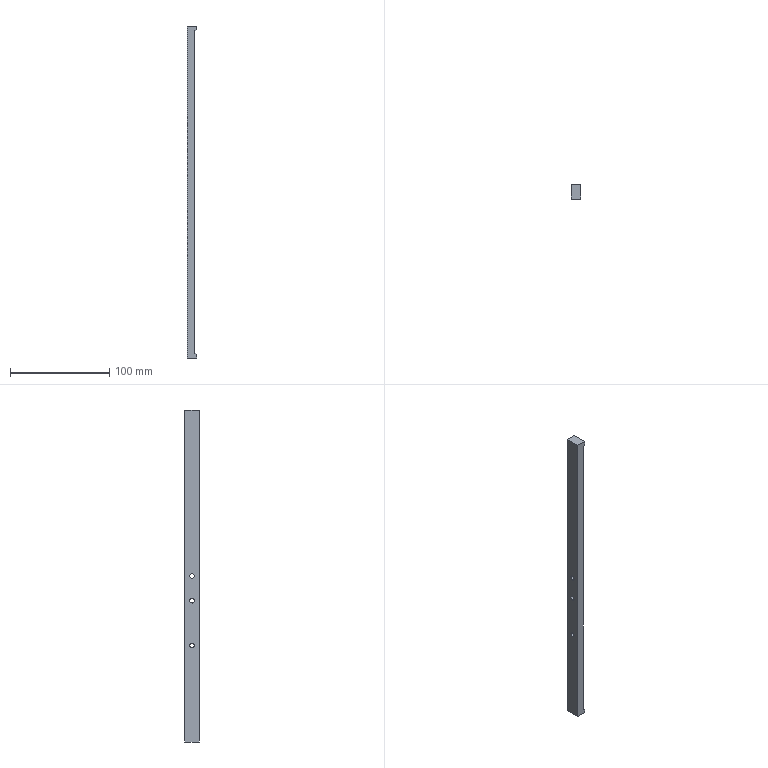Part | SolidWorks | features Extrusion 1, HoleWzd 1, ICE 1 | 1 solid | 25 faces | box 10 x 15 x 335 mm | volume 39599 mm3 | plane 13 | cylinder 12 | commonest cylinder face diameters 4.5 x6 8 x6
STEP:
#1=CARTESIAN_POINT('',(3.4,0.,4.));
#2=VERTEX_POINT('',#1);
#3=CARTESIAN_POINT('',(3.4,0.,-4.));
#4=VERTEX_POINT('',#3);
#5=CARTESIAN_POINT('',(3.4,0.,0.));
#6=DIRECTION('',(1.,0.,0.));
#7=DIRECTION('',(0.,0.,-1.));
#8=AXIS2_PLACEMENT_3D('',#5,#6,#7);
#9=CIRCLE('',#8,4.);
#10=EDGE_CURVE('',#2,#4,#9,.T.);
#11=ORIENTED_EDGE('',*,*,#10,.F.);
#12=CARTESIAN_POINT('',(8.,0.,4.));
#13=VERTEX_POINT('',#12);
#14=CARTESIAN_POINT('',(8.,0.,4.));
#15=DIRECTION('',(1.,0.,0.));
#16=VECTOR('',#15,1000.);
#17=LINE('',#14,#16);
#18=EDGE_CURVE('',#2,#13,#17,.T.);
#19=ORIENTED_EDGE('',*,*,#18,.T.);
#20=CARTESIAN_POINT('',(8.,0.,-4.));
#21=VERTEX_POINT('',#20);
#22=CARTESIAN_POINT('',(8.,0.,0.));
#23=DIRECTION('',(1.,0.,0.));
#24=DIRECTION('',(0.,0.,-1.));
#25=AXIS2_PLACEMENT_3D('',#22,#23,#24);
#26=CIRCLE('',#25,4.);
#27=EDGE_CURVE('',#13,#21,#26,.T.);
#28=ORIENTED_EDGE('',*,*,#27,.T.);
#29=CARTESIAN_POINT('',(8.,0.,-4.));
#30=DIRECTION('',(1.,0.,0.));
#31=VECTOR('',#30,1000.);
#32=LINE('',#29,#31);
#33=EDGE_CURVE('',#4,#21,#32,.T.);
#34=ORIENTED_EDGE('',*,*,#33,.F.);
#35=EDGE_LOOP('',(#11,#19,#28,#34));
#36=FACE_OUTER_BOUND('',#35,.T.);
#37=CARTESIAN_POINT('',(8.,0.,0.));
#38=DIRECTION('',(1.,0.,0.));
#39=DIRECTION('',(0.,0.,-1.));
#40=AXIS2_PLACEMENT_3D('',#37,#38,#39);
#41=CYLINDRICAL_SURFACE('',#40,4.);
#42=ADVANCED_FACE('',(#36),#41,.F.);
#43=CARTESIAN_POINT('',(0.,0.,2.25));
#44=VERTEX_POINT('',#43);
#45=CARTESIAN_POINT('',(0.,0.,-2.25));
#46=VERTEX_POINT('',#45);
#47=CARTESIAN_POINT('',(0.,0.,0.));
#48=DIRECTION('',(1.,0.,0.));
#49=DIRECTION('',(0.,0.,-1.));
#50=AXIS2_PLACEMENT_3D('',#47,#48,#49);
#51=CIRCLE('',#50,2.25);
#52=EDGE_CURVE('',#44,#46,#51,.T.);
#53=ORIENTED_EDGE('',*,*,#52,.F.);
#54=CARTESIAN_POINT('',(3.4,0.,2.25));
#55=VERTEX_POINT('',#54);
#56=CARTESIAN_POINT('',(8.,0.,2.25));
#57=DIRECTION('',(1.,0.,0.));
#58=VECTOR('',#57,1000.);
#59=LINE('',#56,#58);
#60=EDGE_CURVE('',#44,#55,#59,.T.);
#61=ORIENTED_EDGE('',*,*,#60,.T.);
#62=CARTESIAN_POINT('',(3.4,0.,-2.25));
#63=VERTEX_POINT('',#62);
#64=CARTESIAN_POINT('',(3.4,0.,0.));
#65=DIRECTION('',(1.,0.,0.));
#66=DIRECTION('',(0.,0.,-1.));
#67=AXIS2_PLACEMENT_3D('',#64,#65,#66);
#68=CIRCLE('',#67,2.25);
#69=EDGE_CURVE('',#55,#63,#68,.T.);
#70=ORIENTED_EDGE('',*,*,#69,.T.);
#71=CARTESIAN_POINT('',(8.,0.,-2.25));
#72=DIRECTION('',(1.,0.,0.));
#73=VECTOR('',#72,1000.);
#74=LINE('',#71,#73);
#75=EDGE_CURVE('',#46,#63,#74,.T.);
#76=ORIENTED_EDGE('',*,*,#75,.F.);
#77=EDGE_LOOP('',(#53,#61,#70,#76));
#78=FACE_OUTER_BOUND('',#77,.T.);
#79=CARTESIAN_POINT('',(8.,0.,0.));
#80=DIRECTION('',(1.,0.,0.));
#81=DIRECTION('',(0.,0.,-1.));
#82=AXIS2_PLACEMENT_3D('',#79,#80,#81);
#83=CYLINDRICAL_SURFACE('',#82,2.25);
#84=ADVANCED_FACE('',(#78),#83,.F.);
#85=CARTESIAN_POINT('',(3.4,0.,-66.));
#86=VERTEX_POINT('',#85);
#87=CARTESIAN_POINT('',(3.4,0.,-74.));
#88=VERTEX_POINT('',#87);
#89=CARTESIAN_POINT('',(3.4,0.,-70.));
#90=DIRECTION('',(1.,0.,0.));
#91=DIRECTION('',(0.,0.,-1.));
#92=AXIS2_PLACEMENT_3D('',#89,#90,#91);
#93=CIRCLE('',#92,4.);
#94=EDGE_CURVE('',#86,#88,#93,.T.);
#95=ORIENTED_EDGE('',*,*,#94,.F.);
#96=CARTESIAN_POINT('',(8.,0.,-66.));
#97=VERTEX_POINT('',#96);
#98=CARTESIAN_POINT('',(8.,0.,-66.));
#99=DIRECTION('',(1.,0.,0.));
#100=VECTOR('',#99,1000.);
#101=LINE('',#98,#100);
#102=EDGE_CURVE('',#86,#97,#101,.T.);
#103=ORIENTED_EDGE('',*,*,#102,.T.);
#104=CARTESIAN_POINT('',(8.,0.,-74.));
#105=VERTEX_POINT('',#104);
#106=CARTESIAN_POINT('',(8.,0.,-70.));
#107=DIRECTION('',(1.,0.,0.));
#108=DIRECTION('',(0.,0.,-1.));
#109=AXIS2_PLACEMENT_3D('',#106,#107,#108);
#110=CIRCLE('',#109,4.);
#111=EDGE_CURVE('',#97,#105,#110,.T.);
#112=ORIENTED_EDGE('',*,*,#111,.T.);
#113=CARTESIAN_POINT('',(8.,0.,-74.));
#114=DIRECTION('',(1.,0.,0.));
#115=VECTOR('',#114,1000.);
#116=LINE('',#113,#115);
#117=EDGE_CURVE('',#88,#105,#116,.T.);
#118=ORIENTED_EDGE('',*,*,#117,.F.);
#119=EDGE_LOOP('',(#95,#103,#112,#118));
#120=FACE_OUTER_BOUND('',#119,.T.);
#121=CARTESIAN_POINT('',(8.,0.,-70.));
#122=DIRECTION('',(1.,0.,0.));
#123=DIRECTION('',(0.,0.,-1.));
#124=AXIS2_PLACEMENT_3D('',#121,#122,#123);
#125=CYLINDRICAL_SURFACE('',#124,4.);
#126=ADVANCED_FACE('',(#120),#125,.F.);
#127=CARTESIAN_POINT('',(0.,0.,-67.75));
#128=VERTEX_POINT('',#127);
#129=CARTESIAN_POINT('',(0.,0.,-72.25));
#130=VERTEX_POINT('',#129);
#131=CARTESIAN_POINT('',(0.,0.,-70.));
#132=DIRECTION('',(1.,0.,0.));
#133=DIRECTION('',(0.,0.,-1.));
#134=AXIS2_PLACEMENT_3D('',#131,#132,#133);
#135=CIRCLE('',#134,2.25);
#136=EDGE_CURVE('',#128,#130,#135,.T.);
#137=ORIENTED_EDGE('',*,*,#136,.F.);
#138=CARTESIAN_POINT('',(3.4,0.,-67.75));
#139=VERTEX_POINT('',#138);
#140=CARTESIAN_POINT('',(8.,0.,-67.75));
#141=DIRECTION('',(1.,0.,0.));
#142=VECTOR('',#141,1000.);
#143=LINE('',#140,#142);
#144=EDGE_CURVE('',#128,#139,#143,.T.);
#145=ORIENTED_EDGE('',*,*,#144,.T.);
#146=CARTESIAN_POINT('',(3.4,0.,-72.25));
#147=VERTEX_POINT('',#146);
#148=CARTESIAN_POINT('',(3.4,0.,-70.));
#149=DIRECTION('',(1.,0.,0.));
#150=DIRECTION('',(0.,0.,-1.));
#151=AXIS2_PLACEMENT_3D('',#148,#149,#150);
#152=CIRCLE('',#151,2.25);
#153=EDGE_CURVE('',#139,#147,#152,.T.);
#154=ORIENTED_EDGE('',*,*,#153,.T.);
#155=CARTESIAN_POINT('',(8.,0.,-72.25));
#156=DIRECTION('',(1.,0.,0.));
#157=VECTOR('',#156,1000.);
#158=LINE('',#155,#157);
#159=EDGE_CURVE('',#130,#147,#158,.T.);
#160=ORIENTED_EDGE('',*,*,#159,.F.);
#161=EDGE_LOOP('',(#137,#145,#154,#160));
#162=FACE_OUTER_BOUND('',#161,.T.);
#163=CARTESIAN_POINT('',(8.,0.,-70.));
#164=DIRECTION('',(1.,0.,0.));
#165=DIRECTION('',(0.,0.,-1.));
#166=AXIS2_PLACEMENT_3D('',#163,#164,#165);
#167=CYLINDRICAL_SURFACE('',#166,2.25);
#168=ADVANCED_FACE('',(#162),#167,.F.);
#169=CARTESIAN_POINT('',(3.4,0.,-21.));
#170=VERTEX_POINT('',#169);
#171=CARTESIAN_POINT('',(3.4,0.,-29.));
#172=VERTEX_POINT('',#171);
#173=CARTESIAN_POINT('',(3.4,0.,-25.));
#174=DIRECTION('',(1.,0.,0.));
#175=DIRECTION('',(0.,0.,-1.));
#176=AXIS2_PLACEMENT_3D('',#173,#174,#175);
#177=CIRCLE('',#176,4.);
#178=EDGE_CURVE('',#170,#172,#177,.T.);
#179=ORIENTED_EDGE('',*,*,#178,.F.);
#180=CARTESIAN_POINT('',(8.,0.,-21.));
#181=VERTEX_POINT('',#180);
#182=CARTESIAN_POINT('',(8.,0.,-21.));
#183=DIRECTION('',(1.,0.,0.));
#184=VECTOR('',#183,1000.);
#185=LINE('',#182,#184);
#186=EDGE_CURVE('',#170,#181,#185,.T.);
#187=ORIENTED_EDGE('',*,*,#186,.T.);
#188=CARTESIAN_POINT('',(8.,0.,-29.));
#189=VERTEX_POINT('',#188);
#190=CARTESIAN_POINT('',(8.,0.,-25.));
#191=DIRECTION('',(1.,0.,0.));
#192=DIRECTION('',(0.,0.,-1.));
#193=AXIS2_PLACEMENT_3D('',#190,#191,#192);
#194=CIRCLE('',#193,4.);
#195=EDGE_CURVE('',#181,#189,#194,.T.);
#196=ORIENTED_EDGE('',*,*,#195,.T.);
#197=CARTESIAN_POINT('',(8.,0.,-29.));
#198=DIRECTION('',(1.,0.,0.));
#199=VECTOR('',#198,1000.);
#200=LINE('',#197,#199);
#201=EDGE_CURVE('',#172,#189,#200,.T.);
#202=ORIENTED_EDGE('',*,*,#201,.F.);
#203=EDGE_LOOP('',(#179,#187,#196,#202));
#204=FACE_OUTER_BOUND('',#203,.T.);
#205=CARTESIAN_POINT('',(8.,0.,-25.));
#206=DIRECTION('',(1.,0.,0.));
#207=DIRECTION('',(0.,0.,-1.));
#208=AXIS2_PLACEMENT_3D('',#205,#206,#207);
#209=CYLINDRICAL_SURFACE('',#208,4.);
#210=ADVANCED_FACE('',(#204),#209,.F.);
#211=CARTESIAN_POINT('',(0.,0.,-22.75));
#212=VERTEX_POINT('',#211);
#213=CARTESIAN_POINT('',(0.,0.,-27.25));
#214=VERTEX_POINT('',#213);
#215=CARTESIAN_POINT('',(0.,0.,-25.));
#216=DIRECTION('',(1.,0.,0.));
#217=DIRECTION('',(0.,0.,-1.));
#218=AXIS2_PLACEMENT_3D('',#215,#216,#217);
#219=CIRCLE('',#218,2.25);
#220=EDGE_CURVE('',#212,#214,#219,.T.);
#221=ORIENTED_EDGE('',*,*,#220,.F.);
#222=CARTESIAN_POINT('',(3.4,0.,-22.75));
#223=VERTEX_POINT('',#222);
#224=CARTESIAN_POINT('',(8.,0.,-22.75));
#225=DIRECTION('',(1.,0.,0.));
#226=VECTOR('',#225,1000.);
#227=LINE('',#224,#226);
#228=EDGE_CURVE('',#212,#223,#227,.T.);
#229=ORIENTED_EDGE('',*,*,#228,.T.);
#230=CARTESIAN_POINT('',(3.4,0.,-27.25));
#231=VERTEX_POINT('',#230);
#232=CARTESIAN_POINT('',(3.4,0.,-25.));
#233=DIRECTION('',(1.,0.,0.));
#234=DIRECTION('',(0.,0.,-1.));
#235=AXIS2_PLACEMENT_3D('',#232,#233,#234);
#236=CIRCLE('',#235,2.25);
#237=EDGE_CURVE('',#223,#231,#236,.T.);
#238=ORIENTED_EDGE('',*,*,#237,.T.);
#239=CARTESIAN_POINT('',(8.,0.,-27.25));
#240=DIRECTION('',(1.,0.,0.));
#241=VECTOR('',#240,1000.);
#242=LINE('',#239,#241);
#243=EDGE_CURVE('',#214,#231,#242,.T.);
#244=ORIENTED_EDGE('',*,*,#243,.F.);
#245=EDGE_LOOP('',(#221,#229,#238,#244));
#246=FACE_OUTER_BOUND('',#245,.T.);
#247=CARTESIAN_POINT('',(8.,0.,-25.));
#248=DIRECTION('',(1.,0.,0.));
#249=DIRECTION('',(0.,0.,-1.));
#250=AXIS2_PLACEMENT_3D('',#247,#248,#249);
#251=CYLINDRICAL_SURFACE('',#250,2.25);
#252=ADVANCED_FACE('',(#246),#251,.F.);
#253=CARTESIAN_POINT('',(10.,7.5,-167.5));
#254=VERTEX_POINT('',#253);
#255=CARTESIAN_POINT('',(10.,7.5,-164.));
#256=VERTEX_POINT('',#255);
#257=CARTESIAN_POINT('',(10.,7.5,167.5));
#258=DIRECTION('',(0.,0.,1.));
#259=VECTOR('',#258,1000.);
#260=LINE('',#257,#259);
#261=EDGE_CURVE('',#254,#256,#260,.T.);
#262=ORIENTED_EDGE('',*,*,#261,.T.);
#263=CARTESIAN_POINT('',(10.,-7.5,-164.));
#264=VERTEX_POINT('',#263);
#265=CARTESIAN_POINT('',(10.,7.5,-164.));
#266=DIRECTION('',(0.,-1.,0.));
#267=VECTOR('',#266,1000.);
#268=LINE('',#265,#267);
#269=EDGE_CURVE('',#256,#264,#268,.T.);
#270=ORIENTED_EDGE('',*,*,#269,.T.);
#271=CARTESIAN_POINT('',(10.,-7.5,-167.5));
#272=VERTEX_POINT('',#271);
#273=CARTESIAN_POINT('',(10.,-7.5,167.5));
#274=DIRECTION('',(0.,0.,-1.));
#275=VECTOR('',#274,1000.);
#276=LINE('',#273,#275);
#277=EDGE_CURVE('',#264,#272,#276,.T.);
#278=ORIENTED_EDGE('',*,*,#277,.T.);
#279=CARTESIAN_POINT('',(10.,-7.5,-167.5));
#280=DIRECTION('',(0.,1.,0.));
#281=VECTOR('',#280,1000.);
#282=LINE('',#279,#281);
#283=EDGE_CURVE('',#272,#254,#282,.T.);
#284=ORIENTED_EDGE('',*,*,#283,.T.);
#285=EDGE_LOOP('',(#262,#270,#278,#284));
#286=FACE_OUTER_BOUND('',#285,.T.);
#287=CARTESIAN_POINT('',(10.,0.,0.));
#288=DIRECTION('',(-1.,0.,0.));
#289=DIRECTION('',(0.,0.,1.));
#290=AXIS2_PLACEMENT_3D('',#287,#288,#289);
#291=PLANE('',#290);
#292=ADVANCED_FACE('',(#286),#291,.F.);
#293=CARTESIAN_POINT('',(0.,-7.5,-167.5));
#294=VERTEX_POINT('',#293);
#295=CARTESIAN_POINT('',(0.,7.5,-167.5));
#296=VERTEX_POINT('',#295);
#297=CARTESIAN_POINT('',(0.,-7.5,-167.5));
#298=DIRECTION('',(0.,1.,0.));
#299=VECTOR('',#298,1000.);
#300=LINE('',#297,#299);
#301=EDGE_CURVE('',#294,#296,#300,.T.);
#302=ORIENTED_EDGE('',*,*,#301,.T.);
#303=CARTESIAN_POINT('',(10.,7.5,-167.5));
#304=DIRECTION('',(-1.,0.,0.));
#305=VECTOR('',#304,1000.);
#306=LINE('',#303,#305);
#307=EDGE_CURVE('',#254,#296,#306,.T.);
#308=ORIENTED_EDGE('',*,*,#307,.F.);
#309=ORIENTED_EDGE('',*,*,#283,.F.);
#310=CARTESIAN_POINT('',(10.,-7.5,-167.5));
#311=DIRECTION('',(-1.,0.,0.));
#312=VECTOR('',#311,1000.);
#313=LINE('',#310,#312);
#314=EDGE_CURVE('',#272,#294,#313,.T.);
#315=ORIENTED_EDGE('',*,*,#314,.T.);
#316=EDGE_LOOP('',(#302,#308,#309,#315));
#317=FACE_OUTER_BOUND('',#316,.T.);
#318=CARTESIAN_POINT('',(10.,-7.5,-167.5));
#319=DIRECTION('',(0.,0.,1.));
#320=DIRECTION('',(1.,0.,0.));
#321=AXIS2_PLACEMENT_3D('',#318,#319,#320);
#322=PLANE('',#321);
#323=ADVANCED_FACE('',(#317),#322,.F.);
#324=CARTESIAN_POINT('',(8.,7.5,162.5));
#325=VERTEX_POINT('',#324);
#326=CARTESIAN_POINT('',(8.,7.5,-162.5));
#327=VERTEX_POINT('',#326);
#328=CARTESIAN_POINT('',(8.,7.5,162.5));
#329=DIRECTION('',(0.,0.,-1.));
#330=VECTOR('',#329,1000.);
#331=LINE('',#328,#330);
#332=EDGE_CURVE('',#325,#327,#331,.T.);
#333=ORIENTED_EDGE('',*,*,#332,.T.);
#334=CARTESIAN_POINT('',(10.,7.5,-164.));
#335=DIRECTION('',(0.8,0.,-0.6));
#336=VECTOR('',#335,1000.);
#337=LINE('',#334,#336);
#338=EDGE_CURVE('',#327,#256,#337,.T.);
#339=ORIENTED_EDGE('',*,*,#338,.T.);
#340=ORIENTED_EDGE('',*,*,#261,.F.);
#341=ORIENTED_EDGE('',*,*,#307,.T.);
#342=CARTESIAN_POINT('',(0.,7.5,167.5));
#343=VERTEX_POINT('',#342);
#344=CARTESIAN_POINT('',(0.,7.5,167.5));
#345=DIRECTION('',(0.,0.,1.));
#346=VECTOR('',#345,1000.);
#347=LINE('',#344,#346);
#348=EDGE_CURVE('',#296,#343,#347,.T.);
#349=ORIENTED_EDGE('',*,*,#348,.T.);
#350=CARTESIAN_POINT('',(10.,7.5,167.5));
#351=VERTEX_POINT('',#350);
#352=CARTESIAN_POINT('',(10.,7.5,167.5));
#353=DIRECTION('',(-1.,0.,0.));
#354=VECTOR('',#353,1000.);
#355=LINE('',#352,#354);
#356=EDGE_CURVE('',#351,#343,#355,.T.);
#357=ORIENTED_EDGE('',*,*,#356,.F.);
#358=CARTESIAN_POINT('',(10.,7.5,164.));
#359=VERTEX_POINT('',#358);
#360=CARTESIAN_POINT('',(10.,7.5,167.5));
#361=DIRECTION('',(0.,0.,1.));
#362=VECTOR('',#361,1000.);
#363=LINE('',#360,#362);
#364=EDGE_CURVE('',#359,#351,#363,.T.);
#365=ORIENTED_EDGE('',*,*,#364,.F.);
#366=CARTESIAN_POINT('',(10.,7.5,164.));
#367=DIRECTION('',(-0.8,0.,-0.6));
#368=VECTOR('',#367,1000.);
#369=LINE('',#366,#368);
#370=EDGE_CURVE('',#359,#325,#369,.T.);
#371=ORIENTED_EDGE('',*,*,#370,.T.);
#372=EDGE_LOOP('',(#333,#339,#340,#341,#349,#357,#365,#371));
#373=FACE_OUTER_BOUND('',#372,.T.);
#374=CARTESIAN_POINT('',(10.,7.5,167.5));
#375=DIRECTION('',(0.,-1.,0.));
#376=DIRECTION('',(0.,0.,-1.));
#377=AXIS2_PLACEMENT_3D('',#374,#375,#376);
#378=PLANE('',#377);
#379=ADVANCED_FACE('',(#373),#378,.F.);
#380=CARTESIAN_POINT('',(0.,-7.5,167.5));
#381=VERTEX_POINT('',#380);
#382=CARTESIAN_POINT('',(0.,-7.5,167.5));
#383=DIRECTION('',(0.,-1.,0.));
#384=VECTOR('',#383,1000.);
#385=LINE('',#382,#384);
#386=EDGE_CURVE('',#343,#381,#385,.T.);
#387=ORIENTED_EDGE('',*,*,#386,.T.);
#388=CARTESIAN_POINT('',(10.,-7.5,167.5));
#389=VERTEX_POINT('',#388);
#390=CARTESIAN_POINT('',(10.,-7.5,167.5));
#391=DIRECTION('',(-1.,0.,0.));
#392=VECTOR('',#391,1000.);
#393=LINE('',#390,#392);
#394=EDGE_CURVE('',#389,#381,#393,.T.);
#395=ORIENTED_EDGE('',*,*,#394,.F.);
#396=CARTESIAN_POINT('',(10.,-7.5,167.5));
#397=DIRECTION('',(0.,-1.,0.));
#398=VECTOR('',#397,1000.);
#399=LINE('',#396,#398);
#400=EDGE_CURVE('',#351,#389,#399,.T.);
#401=ORIENTED_EDGE('',*,*,#400,.F.);
#402=ORIENTED_EDGE('',*,*,#356,.T.);
#403=EDGE_LOOP('',(#387,#395,#401,#402));
#404=FACE_OUTER_BOUND('',#403,.T.);
#405=CARTESIAN_POINT('',(10.,-7.5,167.5));
#406=DIRECTION('',(0.,0.,-1.));
#407=DIRECTION('',(-1.,0.,0.));
#408=AXIS2_PLACEMENT_3D('',#405,#406,#407);
#409=PLANE('',#408);
#410=ADVANCED_FACE('',(#404),#409,.F.);
#411=ORIENTED_EDGE('',*,*,#277,.F.);
#412=CARTESIAN_POINT('',(8.,-7.5,-162.5));
#413=VERTEX_POINT('',#412);
#414=CARTESIAN_POINT('',(10.,-7.5,-164.));
#415=DIRECTION('',(0.8,0.,-0.6));
#416=VECTOR('',#415,1000.);
#417=LINE('',#414,#416);
#418=EDGE_CURVE('',#413,#264,#417,.T.);
#419=ORIENTED_EDGE('',*,*,#418,.F.);
#420=CARTESIAN_POINT('',(8.,-7.5,162.5));
#421=VERTEX_POINT('',#420);
#422=CARTESIAN_POINT('',(8.,-7.5,162.5));
#423=DIRECTION('',(0.,0.,-1.));
#424=VECTOR('',#423,1000.);
#425=LINE('',#422,#424);
#426=EDGE_CURVE('',#421,#413,#425,.T.);
#427=ORIENTED_EDGE('',*,*,#426,.F.);
#428=CARTESIAN_POINT('',(10.,-7.5,164.));
#429=VERTEX_POINT('',#428);
#430=CARTESIAN_POINT('',(10.,-7.5,164.));
#431=DIRECTION('',(-0.8,0.,-0.6));
#432=VECTOR('',#431,1000.);
#433=LINE('',#430,#432);
#434=EDGE_CURVE('',#429,#421,#433,.T.);
#435=ORIENTED_EDGE('',*,*,#434,.F.);
#436=CARTESIAN_POINT('',(10.,-7.5,167.5));
#437=DIRECTION('',(0.,0.,-1.));
#438=VECTOR('',#437,1000.);
#439=LINE('',#436,#438);
#440=EDGE_CURVE('',#389,#429,#439,.T.);
#441=ORIENTED_EDGE('',*,*,#440,.F.);
#442=ORIENTED_EDGE('',*,*,#394,.T.);
#443=CARTESIAN_POINT('',(0.,-7.5,167.5));
#444=DIRECTION('',(0.,0.,-1.));
#445=VECTOR('',#444,1000.);
#446=LINE('',#443,#445);
#447=EDGE_CURVE('',#381,#294,#446,.T.);
#448=ORIENTED_EDGE('',*,*,#447,.T.);
#449=ORIENTED_EDGE('',*,*,#314,.F.);
#450=EDGE_LOOP('',(#411,#419,#427,#435,#441,#442,#448,#449));
#451=FACE_OUTER_BOUND('',#450,.T.);
#452=CARTESIAN_POINT('',(10.,-7.5,167.5));
#453=DIRECTION('',(0.,1.,0.));
#454=DIRECTION('',(0.,0.,1.));
#455=AXIS2_PLACEMENT_3D('',#452,#453,#454);
#456=PLANE('',#455);
#457=ADVANCED_FACE('',(#451),#456,.F.);
#458=ORIENTED_EDGE('',*,*,#440,.T.);
#459=CARTESIAN_POINT('',(10.,7.5,164.));
#460=DIRECTION('',(0.,-1.,0.));
#461=VECTOR('',#460,1000.);
#462=LINE('',#459,#461);
#463=EDGE_CURVE('',#359,#429,#462,.T.);
#464=ORIENTED_EDGE('',*,*,#463,.F.);
#465=ORIENTED_EDGE('',*,*,#364,.T.);
#466=ORIENTED_EDGE('',*,*,#400,.T.);
#467=EDGE_LOOP('',(#458,#464,#465,#466));
#468=FACE_OUTER_BOUND('',#467,.T.);
#469=CARTESIAN_POINT('',(10.,0.,0.));
#470=DIRECTION('',(-1.,0.,0.));
#471=DIRECTION('',(0.,0.,1.));
#472=AXIS2_PLACEMENT_3D('',#469,#470,#471);
#473=PLANE('',#472);
#474=ADVANCED_FACE('',(#468),#473,.F.);
#475=CARTESIAN_POINT('',(0.,0.,0.));
#476=DIRECTION('',(1.,0.,0.));
#477=DIRECTION('',(0.,0.,-1.));
#478=AXIS2_PLACEMENT_3D('',#475,#476,#477);
#479=CIRCLE('',#478,2.25);
#480=EDGE_CURVE('',#46,#44,#479,.T.);
#481=ORIENTED_EDGE('',*,*,#480,.T.);
#482=ORIENTED_EDGE('',*,*,#52,.T.);
#483=EDGE_LOOP('',(#481,#482));
#484=FACE_BOUND('',#483,.T.);
#485=CARTESIAN_POINT('',(0.,0.,-70.));
#486=DIRECTION('',(1.,0.,0.));
#487=DIRECTION('',(0.,0.,-1.));
#488=AXIS2_PLACEMENT_3D('',#485,#486,#487);
#489=CIRCLE('',#488,2.25);
#490=EDGE_CURVE('',#130,#128,#489,.T.);
#491=ORIENTED_EDGE('',*,*,#490,.T.);
#492=ORIENTED_EDGE('',*,*,#136,.T.);
#493=EDGE_LOOP('',(#491,#492));
#494=FACE_BOUND('',#493,.T.);
#495=CARTESIAN_POINT('',(0.,0.,-25.));
#496=DIRECTION('',(1.,0.,0.));
#497=DIRECTION('',(0.,0.,-1.));
#498=AXIS2_PLACEMENT_3D('',#495,#496,#497);
#499=CIRCLE('',#498,2.25);
#500=EDGE_CURVE('',#214,#212,#499,.T.);
#501=ORIENTED_EDGE('',*,*,#500,.T.);
#502=ORIENTED_EDGE('',*,*,#220,.T.);
#503=EDGE_LOOP('',(#501,#502));
#504=FACE_BOUND('',#503,.T.);
#505=ORIENTED_EDGE('',*,*,#301,.F.);
#506=ORIENTED_EDGE('',*,*,#447,.F.);
#507=ORIENTED_EDGE('',*,*,#386,.F.);
#508=ORIENTED_EDGE('',*,*,#348,.F.);
#509=EDGE_LOOP('',(#505,#506,#507,#508));
#510=FACE_OUTER_BOUND('',#509,.T.);
#511=CARTESIAN_POINT('',(0.,0.,0.));
#512=DIRECTION('',(-1.,0.,0.));
#513=DIRECTION('',(0.,0.,1.));
#514=AXIS2_PLACEMENT_3D('',#511,#512,#513);
#515=PLANE('',#514);
#516=ADVANCED_FACE('',(#484,#494,#504,#510),#515,.T.);
#517=ORIENTED_EDGE('',*,*,#418,.T.);
#518=ORIENTED_EDGE('',*,*,#269,.F.);
#519=ORIENTED_EDGE('',*,*,#338,.F.);
#520=CARTESIAN_POINT('',(8.,7.5,-162.5));
#521=DIRECTION('',(0.,-1.,0.));
#522=VECTOR('',#521,1000.);
#523=LINE('',#520,#522);
#524=EDGE_CURVE('',#327,#413,#523,.T.);
#525=ORIENTED_EDGE('',*,*,#524,.T.);
#526=EDGE_LOOP('',(#517,#518,#519,#525));
#527=FACE_OUTER_BOUND('',#526,.T.);
#528=CARTESIAN_POINT('',(10.,7.5,-164.));
#529=DIRECTION('',(-0.6,0.,-0.8));
#530=DIRECTION('',(-0.8,0.,0.6));
#531=AXIS2_PLACEMENT_3D('',#528,#529,#530);
#532=PLANE('',#531);
#533=ADVANCED_FACE('',(#527),#532,.F.);
#534=CARTESIAN_POINT('',(8.,0.,0.));
#535=DIRECTION('',(1.,0.,0.));
#536=DIRECTION('',(0.,0.,-1.));
#537=AXIS2_PLACEMENT_3D('',#534,#535,#536);
#538=CIRCLE('',#537,4.);
#539=EDGE_CURVE('',#21,#13,#538,.T.);
#540=ORIENTED_EDGE('',*,*,#539,.F.);
#541=ORIENTED_EDGE('',*,*,#27,.F.);
#542=EDGE_LOOP('',(#540,#541));
#543=FACE_BOUND('',#542,.T.);
#544=CARTESIAN_POINT('',(8.,0.,-70.));
#545=DIRECTION('',(1.,0.,0.));
#546=DIRECTION('',(0.,0.,-1.));
#547=AXIS2_PLACEMENT_3D('',#544,#545,#546);
#548=CIRCLE('',#547,4.);
#549=EDGE_CURVE('',#105,#97,#548,.T.);
#550=ORIENTED_EDGE('',*,*,#549,.F.);
#551=ORIENTED_EDGE('',*,*,#111,.F.);
#552=EDGE_LOOP('',(#550,#551));
#553=FACE_BOUND('',#552,.T.);
#554=CARTESIAN_POINT('',(8.,0.,-25.));
#555=DIRECTION('',(1.,0.,0.));
#556=DIRECTION('',(0.,0.,-1.));
#557=AXIS2_PLACEMENT_3D('',#554,#555,#556);
#558=CIRCLE('',#557,4.);
#559=EDGE_CURVE('',#189,#181,#558,.T.);
#560=ORIENTED_EDGE('',*,*,#559,.F.);
#561=ORIENTED_EDGE('',*,*,#195,.F.);
#562=EDGE_LOOP('',(#560,#561));
#563=FACE_BOUND('',#562,.T.);
#564=ORIENTED_EDGE('',*,*,#426,.T.);
#565=ORIENTED_EDGE('',*,*,#524,.F.);
#566=ORIENTED_EDGE('',*,*,#332,.F.);
#567=CARTESIAN_POINT('',(8.,7.5,162.5));
#568=DIRECTION('',(0.,-1.,0.));
#569=VECTOR('',#568,1000.);
#570=LINE('',#567,#569);
#571=EDGE_CURVE('',#325,#421,#570,.T.);
#572=ORIENTED_EDGE('',*,*,#571,.T.);
#573=EDGE_LOOP('',(#564,#565,#566,#572));
#574=FACE_OUTER_BOUND('',#573,.T.);
#575=CARTESIAN_POINT('',(8.,7.5,162.5));
#576=DIRECTION('',(-1.,0.,0.));
#577=DIRECTION('',(0.,0.,1.));
#578=AXIS2_PLACEMENT_3D('',#575,#576,#577);
#579=PLANE('',#578);
#580=ADVANCED_FACE('',(#543,#553,#563,#574),#579,.F.);
#581=ORIENTED_EDGE('',*,*,#434,.T.);
#582=ORIENTED_EDGE('',*,*,#571,.F.);
#583=ORIENTED_EDGE('',*,*,#370,.F.);
#584=ORIENTED_EDGE('',*,*,#463,.T.);
#585=EDGE_LOOP('',(#581,#582,#583,#584));
#586=FACE_OUTER_BOUND('',#585,.T.);
#587=CARTESIAN_POINT('',(10.,7.5,164.));
#588=DIRECTION('',(-0.6,0.,0.8));
#589=DIRECTION('',(0.8,0.,0.6));
#590=AXIS2_PLACEMENT_3D('',#587,#588,#589);
#591=PLANE('',#590);
#592=ADVANCED_FACE('',(#586),#591,.F.);
#593=ORIENTED_EDGE('',*,*,#228,.F.);
#594=ORIENTED_EDGE('',*,*,#500,.F.);
#595=ORIENTED_EDGE('',*,*,#243,.T.);
#596=CARTESIAN_POINT('',(3.4,0.,-25.));
#597=DIRECTION('',(1.,0.,0.));
#598=DIRECTION('',(0.,0.,-1.));
#599=AXIS2_PLACEMENT_3D('',#596,#597,#598);
#600=CIRCLE('',#599,2.25);
#601=EDGE_CURVE('',#231,#223,#600,.T.);
#602=ORIENTED_EDGE('',*,*,#601,.T.);
#603=EDGE_LOOP('',(#593,#594,#595,#602));
#604=FACE_OUTER_BOUND('',#603,.T.);
#605=CARTESIAN_POINT('',(8.,0.,-25.));
#606=DIRECTION('',(1.,0.,0.));
#607=DIRECTION('',(0.,0.,-1.));
#608=AXIS2_PLACEMENT_3D('',#605,#606,#607);
#609=CYLINDRICAL_SURFACE('',#608,2.25);
#610=ADVANCED_FACE('',(#604),#609,.F.);
#611=ORIENTED_EDGE('',*,*,#601,.F.);
#612=ORIENTED_EDGE('',*,*,#237,.F.);
#613=EDGE_LOOP('',(#611,#612));
#614=FACE_BOUND('',#613,.T.);
#615=CARTESIAN_POINT('',(3.4,0.,-25.));
#616=DIRECTION('',(1.,0.,0.));
#617=DIRECTION('',(0.,0.,-1.));
#618=AXIS2_PLACEMENT_3D('',#615,#616,#617);
#619=CIRCLE('',#618,4.);
#620=EDGE_CURVE('',#172,#170,#619,.T.);
#621=ORIENTED_EDGE('',*,*,#620,.T.);
#622=ORIENTED_EDGE('',*,*,#178,.T.);
#623=EDGE_LOOP('',(#621,#622));
#624=FACE_OUTER_BOUND('',#623,.T.);
#625=CARTESIAN_POINT('',(3.4,2.25,-25.));
#626=DIRECTION('',(-1.,0.,0.));
#627=DIRECTION('',(0.,0.,1.));
#628=AXIS2_PLACEMENT_3D('',#625,#626,#627);
#629=PLANE('',#628);
#630=ADVANCED_FACE('',(#614,#624),#629,.F.);
#631=ORIENTED_EDGE('',*,*,#186,.F.);
#632=ORIENTED_EDGE('',*,*,#620,.F.);
#633=ORIENTED_EDGE('',*,*,#201,.T.);
#634=ORIENTED_EDGE('',*,*,#559,.T.);
#635=EDGE_LOOP('',(#631,#632,#633,#634));
#636=FACE_OUTER_BOUND('',#635,.T.);
#637=CARTESIAN_POINT('',(8.,0.,-25.));
#638=DIRECTION('',(1.,0.,0.));
#639=DIRECTION('',(0.,0.,-1.));
#640=AXIS2_PLACEMENT_3D('',#637,#638,#639);
#641=CYLINDRICAL_SURFACE('',#640,4.);
#642=ADVANCED_FACE('',(#636),#641,.F.);
#643=ORIENTED_EDGE('',*,*,#144,.F.);
#644=ORIENTED_EDGE('',*,*,#490,.F.);
#645=ORIENTED_EDGE('',*,*,#159,.T.);
#646=CARTESIAN_POINT('',(3.4,0.,-70.));
#647=DIRECTION('',(1.,0.,0.));
#648=DIRECTION('',(0.,0.,-1.));
#649=AXIS2_PLACEMENT_3D('',#646,#647,#648);
#650=CIRCLE('',#649,2.25);
#651=EDGE_CURVE('',#147,#139,#650,.T.);
#652=ORIENTED_EDGE('',*,*,#651,.T.);
#653=EDGE_LOOP('',(#643,#644,#645,#652));
#654=FACE_OUTER_BOUND('',#653,.T.);
#655=CARTESIAN_POINT('',(8.,0.,-70.));
#656=DIRECTION('',(1.,0.,0.));
#657=DIRECTION('',(0.,0.,-1.));
#658=AXIS2_PLACEMENT_3D('',#655,#656,#657);
#659=CYLINDRICAL_SURFACE('',#658,2.25);
#660=ADVANCED_FACE('',(#654),#659,.F.);
#661=ORIENTED_EDGE('',*,*,#651,.F.);
#662=ORIENTED_EDGE('',*,*,#153,.F.);
#663=EDGE_LOOP('',(#661,#662));
#664=FACE_BOUND('',#663,.T.);
#665=CARTESIAN_POINT('',(3.4,0.,-70.));
#666=DIRECTION('',(1.,0.,0.));
#667=DIRECTION('',(0.,0.,-1.));
#668=AXIS2_PLACEMENT_3D('',#665,#666,#667);
#669=CIRCLE('',#668,4.);
#670=EDGE_CURVE('',#88,#86,#669,.T.);
#671=ORIENTED_EDGE('',*,*,#670,.T.);
#672=ORIENTED_EDGE('',*,*,#94,.T.);
#673=EDGE_LOOP('',(#671,#672));
#674=FACE_OUTER_BOUND('',#673,.T.);
#675=CARTESIAN_POINT('',(3.4,2.25,-70.));
#676=DIRECTION('',(-1.,0.,0.));
#677=DIRECTION('',(0.,0.,1.));
#678=AXIS2_PLACEMENT_3D('',#675,#676,#677);
#679=PLANE('',#678);
#680=ADVANCED_FACE('',(#664,#674),#679,.F.);
#681=ORIENTED_EDGE('',*,*,#102,.F.);
#682=ORIENTED_EDGE('',*,*,#670,.F.);
#683=ORIENTED_EDGE('',*,*,#117,.T.);
#684=ORIENTED_EDGE('',*,*,#549,.T.);
#685=EDGE_LOOP('',(#681,#682,#683,#684));
#686=FACE_OUTER_BOUND('',#685,.T.);
#687=CARTESIAN_POINT('',(8.,0.,-70.));
#688=DIRECTION('',(1.,0.,0.));
#689=DIRECTION('',(0.,0.,-1.));
#690=AXIS2_PLACEMENT_3D('',#687,#688,#689);
#691=CYLINDRICAL_SURFACE('',#690,4.);
#692=ADVANCED_FACE('',(#686),#691,.F.);
#693=ORIENTED_EDGE('',*,*,#60,.F.);
#694=ORIENTED_EDGE('',*,*,#480,.F.);
#695=ORIENTED_EDGE('',*,*,#75,.T.);
#696=CARTESIAN_POINT('',(3.4,0.,0.));
#697=DIRECTION('',(1.,0.,0.));
#698=DIRECTION('',(0.,0.,-1.));
#699=AXIS2_PLACEMENT_3D('',#696,#697,#698);
#700=CIRCLE('',#699,2.25);
#701=EDGE_CURVE('',#63,#55,#700,.T.);
#702=ORIENTED_EDGE('',*,*,#701,.T.);
#703=EDGE_LOOP('',(#693,#694,#695,#702));
#704=FACE_OUTER_BOUND('',#703,.T.);
#705=CARTESIAN_POINT('',(8.,0.,0.));
#706=DIRECTION('',(1.,0.,0.));
#707=DIRECTION('',(0.,0.,-1.));
#708=AXIS2_PLACEMENT_3D('',#705,#706,#707);
#709=CYLINDRICAL_SURFACE('',#708,2.25);
#710=ADVANCED_FACE('',(#704),#709,.F.);
#711=ORIENTED_EDGE('',*,*,#701,.F.);
#712=ORIENTED_EDGE('',*,*,#69,.F.);
#713=EDGE_LOOP('',(#711,#712));
#714=FACE_BOUND('',#713,.T.);
#715=CARTESIAN_POINT('',(3.4,0.,0.));
#716=DIRECTION('',(1.,0.,0.));
#717=DIRECTION('',(0.,0.,-1.));
#718=AXIS2_PLACEMENT_3D('',#715,#716,#717);
#719=CIRCLE('',#718,4.);
#720=EDGE_CURVE('',#4,#2,#719,.T.);
#721=ORIENTED_EDGE('',*,*,#720,.T.);
#722=ORIENTED_EDGE('',*,*,#10,.T.);
#723=EDGE_LOOP('',(#721,#722));
#724=FACE_OUTER_BOUND('',#723,.T.);
#725=CARTESIAN_POINT('',(3.4,2.25,0.));
#726=DIRECTION('',(-1.,0.,0.));
#727=DIRECTION('',(0.,0.,1.));
#728=AXIS2_PLACEMENT_3D('',#725,#726,#727);
#729=PLANE('',#728);
#730=ADVANCED_FACE('',(#714,#724),#729,.F.);
#731=ORIENTED_EDGE('',*,*,#18,.F.);
#732=ORIENTED_EDGE('',*,*,#720,.F.);
#733=ORIENTED_EDGE('',*,*,#33,.T.);
#734=ORIENTED_EDGE('',*,*,#539,.T.);
#735=EDGE_LOOP('',(#731,#732,#733,#734));
#736=FACE_OUTER_BOUND('',#735,.T.);
#737=CARTESIAN_POINT('',(8.,0.,0.));
#738=DIRECTION('',(1.,0.,0.));
#739=DIRECTION('',(0.,0.,-1.));
#740=AXIS2_PLACEMENT_3D('',#737,#738,#739);
#741=CYLINDRICAL_SURFACE('',#740,4.);
#742=ADVANCED_FACE('',(#736),#741,.F.);
#743=CLOSED_SHELL('',(#42,#84,#126,#168,#210,#252,#292,#323,#379,#410,#457,#474,#516,#533,#580,#592,#610,#630,#642,#660,#680,#692,#710,#730,#742));
#744=MANIFOLD_SOLID_BREP('',#743);
#745=CARTESIAN_POINT('',(0.,0.,0.));
#746=DIRECTION('',(0.,0.,1.));
#747=DIRECTION('',(1.,0.,0.));
#748=AXIS2_PLACEMENT_3D('',#745,#746,#747);
#749=(LENGTH_UNIT()NAMED_UNIT(*)SI_UNIT(.MILLI.,.METRE.));
#750=UNCERTAINTY_MEASURE_WITH_UNIT(LENGTH_MEASURE(0.00001),#749,'','');
#751=(NAMED_UNIT(*)PLANE_ANGLE_UNIT()SI_UNIT($,.RADIAN.));
#752=(NAMED_UNIT(*)SI_UNIT($,.STERADIAN.)SOLID_ANGLE_UNIT());
#753=(GEOMETRIC_REPRESENTATION_CONTEXT(3)GLOBAL_UNCERTAINTY_ASSIGNED_CONTEXT((#750))GLOBAL_UNIT_ASSIGNED_CONTEXT((#749,#751,#752))REPRESENTATION_CONTEXT('',''));
#754=ADVANCED_BREP_SHAPE_REPRESENTATION('',(#744,#748),#753);